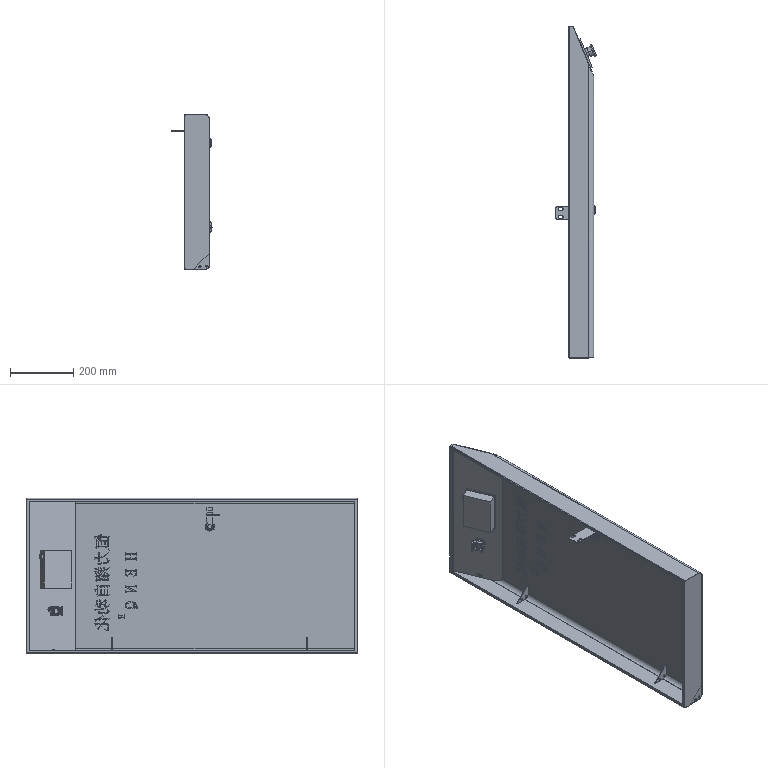Part | SolidWorks | features AEMSimFeature 1, MirrorCompFeat 1 | 10 solids | 786 faces | box 127.543 x 1053 x 493 mm | volume 1598886 mm3 | plane 521 | spline 138 | cylinder 101 | cone 22 | torus 4 | commonest cylinder face diameters 7 x10 6 x8 22 x8 30 x7 6.2 x6 8.3 x6